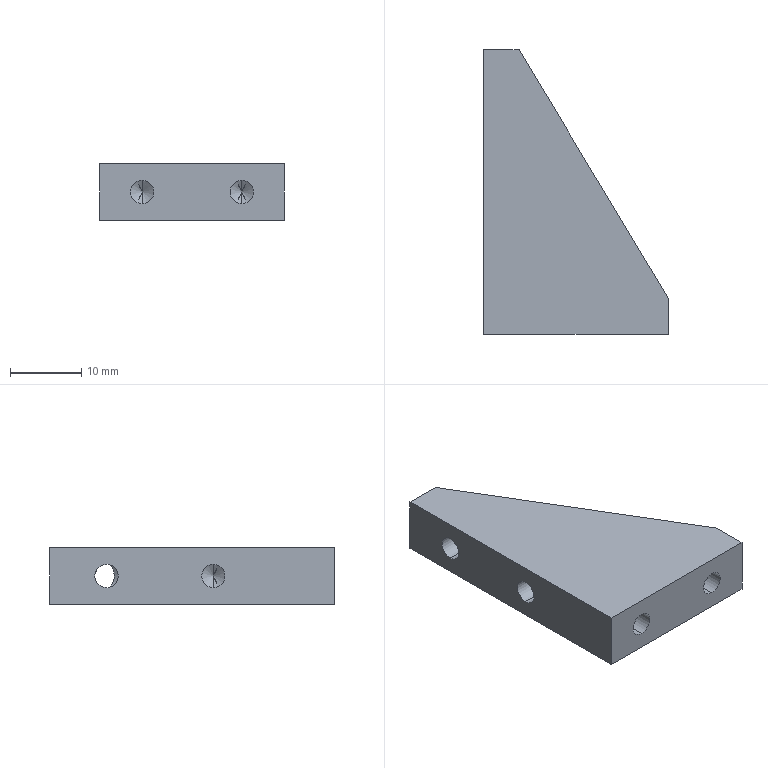Part | STEP file | FBDS-TL-006 | 1 solid | 22 faces | box 26 x 40 x 8 mm | volume 5029 mm3 | cylinder 8 | cone 7 | plane 7 | commonest cylinder face diameters 3.3 x8
STEP:
#1=CARTESIAN_POINT('',(20.,10.1,5.65));
#2=VERTEX_POINT('',#1);
#3=CARTESIAN_POINT('',(20.,10.1,2.35));
#4=VERTEX_POINT('',#3);
#5=CARTESIAN_POINT('',(20.,10.1,4.));
#6=DIRECTION('',(0.,-1.,0.));
#7=DIRECTION('',(0.,0.,-1.));
#8=AXIS2_PLACEMENT_3D('',#5,#6,#7);
#9=CIRCLE('',#8,1.65);
#10=EDGE_CURVE('',#2,#4,#9,.T.);
#11=ORIENTED_EDGE('',*,*,#10,.F.);
#12=CARTESIAN_POINT('',(20.,0.,5.65));
#13=VERTEX_POINT('',#12);
#14=CARTESIAN_POINT('',(20.,0.,5.65));
#15=DIRECTION('',(0.,-1.,0.));
#16=VECTOR('',#15,1000.);
#17=LINE('',#14,#16);
#18=EDGE_CURVE('',#2,#13,#17,.T.);
#19=ORIENTED_EDGE('',*,*,#18,.T.);
#20=CARTESIAN_POINT('',(20.,0.,2.35));
#21=VERTEX_POINT('',#20);
#22=CARTESIAN_POINT('',(20.,0.,4.));
#23=DIRECTION('',(0.,-1.,0.));
#24=DIRECTION('',(0.,0.,-1.));
#25=AXIS2_PLACEMENT_3D('',#22,#23,#24);
#26=CIRCLE('',#25,1.65);
#27=EDGE_CURVE('',#13,#21,#26,.T.);
#28=ORIENTED_EDGE('',*,*,#27,.T.);
#29=CARTESIAN_POINT('',(20.,0.,2.35));
#30=DIRECTION('',(0.,-1.,0.));
#31=VECTOR('',#30,1000.);
#32=LINE('',#29,#31);
#33=EDGE_CURVE('',#4,#21,#32,.T.);
#34=ORIENTED_EDGE('',*,*,#33,.F.);
#35=EDGE_LOOP('',(#11,#19,#28,#34));
#36=FACE_OUTER_BOUND('',#35,.T.);
#37=CARTESIAN_POINT('',(20.,0.,4.));
#38=DIRECTION('',(0.,-1.,0.));
#39=DIRECTION('',(0.,0.,-1.));
#40=AXIS2_PLACEMENT_3D('',#37,#38,#39);
#41=CYLINDRICAL_SURFACE('',#40,1.65);
#42=ADVANCED_FACE('',(#36),#41,.F.);
#43=CARTESIAN_POINT('',(20.,11.091,4.));
#44=VERTEX_POINT('',#43);
#45=CARTESIAN_POINT('',(20.,10.1,2.35));
#46=DIRECTION('',(0.,-0.515,-0.8572));
#47=VECTOR('',#46,1000.);
#48=LINE('',#45,#47);
#49=EDGE_CURVE('',#44,#4,#48,.T.);
#50=ORIENTED_EDGE('',*,*,#49,.F.);
#51=CARTESIAN_POINT('',(20.,10.1,5.65));
#52=DIRECTION('',(0.,-0.515,0.8572));
#53=VECTOR('',#52,1000.);
#54=LINE('',#51,#53);
#55=EDGE_CURVE('',#44,#2,#54,.T.);
#56=ORIENTED_EDGE('',*,*,#55,.T.);
#57=ORIENTED_EDGE('',*,*,#10,.T.);
#58=EDGE_LOOP('',(#50,#56,#57));
#59=FACE_OUTER_BOUND('',#58,.T.);
#60=CARTESIAN_POINT('',(20.,10.1,4.));
#61=DIRECTION('',(0.,-1.,0.));
#62=DIRECTION('',(0.,0.,-1.));
#63=AXIS2_PLACEMENT_3D('',#60,#61,#62);
#64=CONICAL_SURFACE('',#63,1.65,1.03);
#65=ADVANCED_FACE('',(#59),#64,.F.);
#66=CARTESIAN_POINT('',(6.,10.1,5.65));
#67=VERTEX_POINT('',#66);
#68=CARTESIAN_POINT('',(6.,10.1,2.35));
#69=VERTEX_POINT('',#68);
#70=CARTESIAN_POINT('',(6.,10.1,4.));
#71=DIRECTION('',(0.,-1.,0.));
#72=DIRECTION('',(0.,0.,-1.));
#73=AXIS2_PLACEMENT_3D('',#70,#71,#72);
#74=CIRCLE('',#73,1.65);
#75=EDGE_CURVE('',#67,#69,#74,.T.);
#76=ORIENTED_EDGE('',*,*,#75,.F.);
#77=CARTESIAN_POINT('',(6.,0.,5.65));
#78=VERTEX_POINT('',#77);
#79=CARTESIAN_POINT('',(6.,0.,5.65));
#80=DIRECTION('',(0.,-1.,0.));
#81=VECTOR('',#80,1000.);
#82=LINE('',#79,#81);
#83=EDGE_CURVE('',#67,#78,#82,.T.);
#84=ORIENTED_EDGE('',*,*,#83,.T.);
#85=CARTESIAN_POINT('',(6.,0.,2.35));
#86=VERTEX_POINT('',#85);
#87=CARTESIAN_POINT('',(6.,0.,4.));
#88=DIRECTION('',(0.,-1.,0.));
#89=DIRECTION('',(0.,0.,-1.));
#90=AXIS2_PLACEMENT_3D('',#87,#88,#89);
#91=CIRCLE('',#90,1.65);
#92=EDGE_CURVE('',#78,#86,#91,.T.);
#93=ORIENTED_EDGE('',*,*,#92,.T.);
#94=CARTESIAN_POINT('',(6.,0.,2.35));
#95=DIRECTION('',(0.,-1.,0.));
#96=VECTOR('',#95,1000.);
#97=LINE('',#94,#96);
#98=EDGE_CURVE('',#69,#86,#97,.T.);
#99=ORIENTED_EDGE('',*,*,#98,.F.);
#100=EDGE_LOOP('',(#76,#84,#93,#99));
#101=FACE_OUTER_BOUND('',#100,.T.);
#102=CARTESIAN_POINT('',(6.,0.,4.));
#103=DIRECTION('',(0.,-1.,0.));
#104=DIRECTION('',(0.,0.,-1.));
#105=AXIS2_PLACEMENT_3D('',#102,#103,#104);
#106=CYLINDRICAL_SURFACE('',#105,1.65);
#107=ADVANCED_FACE('',(#101),#106,.F.);
#108=CARTESIAN_POINT('',(6.,11.091,4.));
#109=VERTEX_POINT('',#108);
#110=CARTESIAN_POINT('',(6.,10.1,2.35));
#111=DIRECTION('',(0.,-0.515,-0.8572));
#112=VECTOR('',#111,1000.);
#113=LINE('',#110,#112);
#114=EDGE_CURVE('',#109,#69,#113,.T.);
#115=ORIENTED_EDGE('',*,*,#114,.F.);
#116=CARTESIAN_POINT('',(6.,10.1,5.65));
#117=DIRECTION('',(0.,-0.515,0.8572));
#118=VECTOR('',#117,1000.);
#119=LINE('',#116,#118);
#120=EDGE_CURVE('',#109,#67,#119,.T.);
#121=ORIENTED_EDGE('',*,*,#120,.T.);
#122=ORIENTED_EDGE('',*,*,#75,.T.);
#123=EDGE_LOOP('',(#115,#121,#122));
#124=FACE_OUTER_BOUND('',#123,.T.);
#125=CARTESIAN_POINT('',(6.,10.1,4.));
#126=DIRECTION('',(0.,-1.,0.));
#127=DIRECTION('',(0.,0.,-1.));
#128=AXIS2_PLACEMENT_3D('',#125,#126,#127);
#129=CONICAL_SURFACE('',#128,1.65,1.03);
#130=ADVANCED_FACE('',(#124),#129,.F.);
#131=CARTESIAN_POINT('',(9.8,32.,2.35));
#132=VERTEX_POINT('',#131);
#133=CARTESIAN_POINT('',(10.1,31.5,2.428));
#134=VERTEX_POINT('',#133);
#135=CARTESIAN_POINT('',(9.8,32.,2.35));
#136=CARTESIAN_POINT('',(9.902,31.83,2.35));
#137=CARTESIAN_POINT('',(10.003,31.662,2.376));
#138=CARTESIAN_POINT('',(10.1,31.5,2.428));
#139=(BOUNDED_CURVE()B_SPLINE_CURVE(3,(#135,#136,#137,#138),.UNSPECIFIED.,.F.,.F.)B_SPLINE_CURVE_WITH_KNOTS((4,4),(1.571,1.879),.UNSPECIFIED.)CURVE()GEOMETRIC_REPRESENTATION_ITEM()RATIONAL_B_SPLINE_CURVE((1.,0.9921,0.9921,1.))REPRESENTATION_ITEM(''));
#140=EDGE_CURVE('',#132,#134,#139,.T.);
#141=ORIENTED_EDGE('',*,*,#140,.F.);
#142=CARTESIAN_POINT('',(0.,32.,2.35));
#143=VERTEX_POINT('',#142);
#144=CARTESIAN_POINT('',(0.,32.,2.35));
#145=DIRECTION('',(-1.,0.,0.));
#146=VECTOR('',#145,1000.);
#147=LINE('',#144,#146);
#148=EDGE_CURVE('',#132,#143,#147,.T.);
#149=ORIENTED_EDGE('',*,*,#148,.T.);
#150=CARTESIAN_POINT('',(0.,32.,5.65));
#151=VERTEX_POINT('',#150);
#152=CARTESIAN_POINT('',(0.,32.,4.));
#153=DIRECTION('',(-1.,0.,0.));
#154=DIRECTION('',(0.,0.,1.));
#155=AXIS2_PLACEMENT_3D('',#152,#153,#154);
#156=CIRCLE('',#155,1.65);
#157=EDGE_CURVE('',#143,#151,#156,.T.);
#158=ORIENTED_EDGE('',*,*,#157,.T.);
#159=CARTESIAN_POINT('',(9.8,32.,5.65));
#160=VERTEX_POINT('',#159);
#161=CARTESIAN_POINT('',(0.,32.,5.65));
#162=DIRECTION('',(-1.,0.,0.));
#163=VECTOR('',#162,1000.);
#164=LINE('',#161,#163);
#165=EDGE_CURVE('',#160,#151,#164,.T.);
#166=ORIENTED_EDGE('',*,*,#165,.F.);
#167=CARTESIAN_POINT('',(10.1,31.5,5.572));
#168=VERTEX_POINT('',#167);
#169=CARTESIAN_POINT('',(10.1,31.5,5.572));
#170=CARTESIAN_POINT('',(10.003,31.662,5.624));
#171=CARTESIAN_POINT('',(9.902,31.83,5.65));
#172=CARTESIAN_POINT('',(9.8,32.,5.65));
#173=(BOUNDED_CURVE()B_SPLINE_CURVE(3,(#169,#170,#171,#172),.UNSPECIFIED.,.F.,.F.)B_SPLINE_CURVE_WITH_KNOTS((4,4),(4.405,4.712),.UNSPECIFIED.)CURVE()GEOMETRIC_REPRESENTATION_ITEM()RATIONAL_B_SPLINE_CURVE((1.,0.9921,0.9921,1.))REPRESENTATION_ITEM(''));
#174=EDGE_CURVE('',#168,#160,#173,.T.);
#175=ORIENTED_EDGE('',*,*,#174,.F.);
#176=CARTESIAN_POINT('',(10.1,32.,4.));
#177=DIRECTION('',(-1.,0.,0.));
#178=DIRECTION('',(0.,0.,1.));
#179=AXIS2_PLACEMENT_3D('',#176,#177,#178);
#180=CIRCLE('',#179,1.65);
#181=EDGE_CURVE('',#134,#168,#180,.T.);
#182=ORIENTED_EDGE('',*,*,#181,.F.);
#183=EDGE_LOOP('',(#141,#149,#158,#166,#175,#182));
#184=FACE_OUTER_BOUND('',#183,.T.);
#185=CARTESIAN_POINT('',(0.,32.,4.));
#186=DIRECTION('',(-1.,0.,0.));
#187=DIRECTION('',(0.,0.,1.));
#188=AXIS2_PLACEMENT_3D('',#185,#186,#187);
#189=CYLINDRICAL_SURFACE('',#188,1.65);
#190=ADVANCED_FACE('',(#184),#189,.F.);
#191=CARTESIAN_POINT('',(10.1,17.,2.35));
#192=VERTEX_POINT('',#191);
#193=CARTESIAN_POINT('',(10.1,17.,5.65));
#194=VERTEX_POINT('',#193);
#195=CARTESIAN_POINT('',(10.1,17.,4.));
#196=DIRECTION('',(-1.,0.,0.));
#197=DIRECTION('',(0.,0.,1.));
#198=AXIS2_PLACEMENT_3D('',#195,#196,#197);
#199=CIRCLE('',#198,1.65);
#200=EDGE_CURVE('',#192,#194,#199,.T.);
#201=ORIENTED_EDGE('',*,*,#200,.F.);
#202=CARTESIAN_POINT('',(0.,17.,2.35));
#203=VERTEX_POINT('',#202);
#204=CARTESIAN_POINT('',(0.,17.,2.35));
#205=DIRECTION('',(-1.,0.,0.));
#206=VECTOR('',#205,1000.);
#207=LINE('',#204,#206);
#208=EDGE_CURVE('',#192,#203,#207,.T.);
#209=ORIENTED_EDGE('',*,*,#208,.T.);
#210=CARTESIAN_POINT('',(0.,17.,5.65));
#211=VERTEX_POINT('',#210);
#212=CARTESIAN_POINT('',(0.,17.,4.));
#213=DIRECTION('',(-1.,0.,0.));
#214=DIRECTION('',(0.,0.,1.));
#215=AXIS2_PLACEMENT_3D('',#212,#213,#214);
#216=CIRCLE('',#215,1.65);
#217=EDGE_CURVE('',#203,#211,#216,.T.);
#218=ORIENTED_EDGE('',*,*,#217,.T.);
#219=CARTESIAN_POINT('',(0.,17.,5.65));
#220=DIRECTION('',(-1.,0.,0.));
#221=VECTOR('',#220,1000.);
#222=LINE('',#219,#221);
#223=EDGE_CURVE('',#194,#211,#222,.T.);
#224=ORIENTED_EDGE('',*,*,#223,.F.);
#225=EDGE_LOOP('',(#201,#209,#218,#224));
#226=FACE_OUTER_BOUND('',#225,.T.);
#227=CARTESIAN_POINT('',(0.,17.,4.));
#228=DIRECTION('',(-1.,0.,0.));
#229=DIRECTION('',(0.,0.,1.));
#230=AXIS2_PLACEMENT_3D('',#227,#228,#229);
#231=CYLINDRICAL_SURFACE('',#230,1.65);
#232=ADVANCED_FACE('',(#226),#231,.F.);
#233=CARTESIAN_POINT('',(11.091,17.,4.));
#234=VERTEX_POINT('',#233);
#235=CARTESIAN_POINT('',(10.1,17.,5.65));
#236=DIRECTION('',(-0.515,0.,0.8572));
#237=VECTOR('',#236,1000.);
#238=LINE('',#235,#237);
#239=EDGE_CURVE('',#234,#194,#238,.T.);
#240=ORIENTED_EDGE('',*,*,#239,.F.);
#241=CARTESIAN_POINT('',(10.1,17.,2.35));
#242=DIRECTION('',(-0.515,0.,-0.8572));
#243=VECTOR('',#242,1000.);
#244=LINE('',#241,#243);
#245=EDGE_CURVE('',#234,#192,#244,.T.);
#246=ORIENTED_EDGE('',*,*,#245,.T.);
#247=ORIENTED_EDGE('',*,*,#200,.T.);
#248=EDGE_LOOP('',(#240,#246,#247));
#249=FACE_OUTER_BOUND('',#248,.T.);
#250=CARTESIAN_POINT('',(10.1,17.,4.));
#251=DIRECTION('',(-1.,0.,0.));
#252=DIRECTION('',(0.,0.,1.));
#253=AXIS2_PLACEMENT_3D('',#250,#251,#252);
#254=CONICAL_SURFACE('',#253,1.65,1.03);
#255=ADVANCED_FACE('',(#249),#254,.F.);
#256=CARTESIAN_POINT('',(0.,32.,4.));
#257=DIRECTION('',(-1.,0.,0.));
#258=DIRECTION('',(0.,0.,1.));
#259=AXIS2_PLACEMENT_3D('',#256,#257,#258);
#260=CIRCLE('',#259,1.65);
#261=EDGE_CURVE('',#151,#143,#260,.T.);
#262=ORIENTED_EDGE('',*,*,#261,.F.);
#263=ORIENTED_EDGE('',*,*,#157,.F.);
#264=EDGE_LOOP('',(#262,#263));
#265=FACE_BOUND('',#264,.T.);
#266=CARTESIAN_POINT('',(0.,17.,4.));
#267=DIRECTION('',(-1.,0.,0.));
#268=DIRECTION('',(0.,0.,1.));
#269=AXIS2_PLACEMENT_3D('',#266,#267,#268);
#270=CIRCLE('',#269,1.65);
#271=EDGE_CURVE('',#211,#203,#270,.T.);
#272=ORIENTED_EDGE('',*,*,#271,.F.);
#273=ORIENTED_EDGE('',*,*,#217,.F.);
#274=EDGE_LOOP('',(#272,#273));
#275=FACE_BOUND('',#274,.T.);
#276=CARTESIAN_POINT('',(0.,40.,0.));
#277=VERTEX_POINT('',#276);
#278=CARTESIAN_POINT('',(0.,0.,0.));
#279=VERTEX_POINT('',#278);
#280=CARTESIAN_POINT('',(0.,40.,0.));
#281=DIRECTION('',(0.,-1.,0.));
#282=VECTOR('',#281,1000.);
#283=LINE('',#280,#282);
#284=EDGE_CURVE('',#277,#279,#283,.T.);
#285=ORIENTED_EDGE('',*,*,#284,.T.);
#286=CARTESIAN_POINT('',(0.,0.,8.));
#287=VERTEX_POINT('',#286);
#288=CARTESIAN_POINT('',(0.,0.,8.));
#289=DIRECTION('',(0.,0.,-1.));
#290=VECTOR('',#289,1000.);
#291=LINE('',#288,#290);
#292=EDGE_CURVE('',#287,#279,#291,.T.);
#293=ORIENTED_EDGE('',*,*,#292,.F.);
#294=CARTESIAN_POINT('',(0.,40.,8.));
#295=VERTEX_POINT('',#294);
#296=CARTESIAN_POINT('',(0.,40.,8.));
#297=DIRECTION('',(0.,-1.,0.));
#298=VECTOR('',#297,1000.);
#299=LINE('',#296,#298);
#300=EDGE_CURVE('',#295,#287,#299,.T.);
#301=ORIENTED_EDGE('',*,*,#300,.F.);
#302=CARTESIAN_POINT('',(0.,40.,8.));
#303=DIRECTION('',(0.,0.,-1.));
#304=VECTOR('',#303,1000.);
#305=LINE('',#302,#304);
#306=EDGE_CURVE('',#295,#277,#305,.T.);
#307=ORIENTED_EDGE('',*,*,#306,.T.);
#308=EDGE_LOOP('',(#285,#293,#301,#307));
#309=FACE_OUTER_BOUND('',#308,.T.);
#310=CARTESIAN_POINT('',(0.,40.,8.));
#311=DIRECTION('',(1.,0.,0.));
#312=DIRECTION('',(0.,1.,0.));
#313=AXIS2_PLACEMENT_3D('',#310,#311,#312);
#314=PLANE('',#313);
#315=ADVANCED_FACE('',(#265,#275,#309),#314,.F.);
#316=CARTESIAN_POINT('',(20.,0.,4.));
#317=DIRECTION('',(0.,-1.,0.));
#318=DIRECTION('',(0.,0.,-1.));
#319=AXIS2_PLACEMENT_3D('',#316,#317,#318);
#320=CIRCLE('',#319,1.65);
#321=EDGE_CURVE('',#21,#13,#320,.T.);
#322=ORIENTED_EDGE('',*,*,#321,.F.);
#323=ORIENTED_EDGE('',*,*,#27,.F.);
#324=EDGE_LOOP('',(#322,#323));
#325=FACE_BOUND('',#324,.T.);
#326=CARTESIAN_POINT('',(6.,0.,4.));
#327=DIRECTION('',(0.,-1.,0.));
#328=DIRECTION('',(0.,0.,-1.));
#329=AXIS2_PLACEMENT_3D('',#326,#327,#328);
#330=CIRCLE('',#329,1.65);
#331=EDGE_CURVE('',#86,#78,#330,.T.);
#332=ORIENTED_EDGE('',*,*,#331,.F.);
#333=ORIENTED_EDGE('',*,*,#92,.F.);
#334=EDGE_LOOP('',(#332,#333));
#335=FACE_BOUND('',#334,.T.);
#336=CARTESIAN_POINT('',(26.,0.,0.));
#337=VERTEX_POINT('',#336);
#338=CARTESIAN_POINT('',(0.,0.,0.));
#339=DIRECTION('',(1.,0.,0.));
#340=VECTOR('',#339,1000.);
#341=LINE('',#338,#340);
#342=EDGE_CURVE('',#279,#337,#341,.T.);
#343=ORIENTED_EDGE('',*,*,#342,.T.);
#344=CARTESIAN_POINT('',(26.,0.,8.));
#345=VERTEX_POINT('',#344);
#346=CARTESIAN_POINT('',(26.,0.,8.));
#347=DIRECTION('',(0.,0.,-1.));
#348=VECTOR('',#347,1000.);
#349=LINE('',#346,#348);
#350=EDGE_CURVE('',#345,#337,#349,.T.);
#351=ORIENTED_EDGE('',*,*,#350,.F.);
#352=CARTESIAN_POINT('',(0.,0.,8.));
#353=DIRECTION('',(1.,0.,0.));
#354=VECTOR('',#353,1000.);
#355=LINE('',#352,#354);
#356=EDGE_CURVE('',#287,#345,#355,.T.);
#357=ORIENTED_EDGE('',*,*,#356,.F.);
#358=ORIENTED_EDGE('',*,*,#292,.T.);
#359=EDGE_LOOP('',(#343,#351,#357,#358));
#360=FACE_OUTER_BOUND('',#359,.T.);
#361=CARTESIAN_POINT('',(0.,0.,8.));
#362=DIRECTION('',(0.,1.,0.));
#363=DIRECTION('',(0.,0.,1.));
#364=AXIS2_PLACEMENT_3D('',#361,#362,#363);
#365=PLANE('',#364);
#366=ADVANCED_FACE('',(#325,#335,#360),#365,.F.);
#367=CARTESIAN_POINT('',(26.,5.,0.));
#368=VERTEX_POINT('',#367);
#369=CARTESIAN_POINT('',(26.,0.,0.));
#370=DIRECTION('',(0.,1.,0.));
#371=VECTOR('',#370,1000.);
#372=LINE('',#369,#371);
#373=EDGE_CURVE('',#337,#368,#372,.T.);
#374=ORIENTED_EDGE('',*,*,#373,.T.);
#375=CARTESIAN_POINT('',(26.,5.,8.));
#376=VERTEX_POINT('',#375);
#377=CARTESIAN_POINT('',(26.,5.,8.));
#378=DIRECTION('',(0.,0.,-1.));
#379=VECTOR('',#378,1000.);
#380=LINE('',#377,#379);
#381=EDGE_CURVE('',#376,#368,#380,.T.);
#382=ORIENTED_EDGE('',*,*,#381,.F.);
#383=CARTESIAN_POINT('',(26.,0.,8.));
#384=DIRECTION('',(0.,1.,0.));
#385=VECTOR('',#384,1000.);
#386=LINE('',#383,#385);
#387=EDGE_CURVE('',#345,#376,#386,.T.);
#388=ORIENTED_EDGE('',*,*,#387,.F.);
#389=ORIENTED_EDGE('',*,*,#350,.T.);
#390=EDGE_LOOP('',(#374,#382,#388,#389));
#391=FACE_OUTER_BOUND('',#390,.T.);
#392=CARTESIAN_POINT('',(26.,0.,8.));
#393=DIRECTION('',(-1.,0.,0.));
#394=DIRECTION('',(0.,0.,1.));
#395=AXIS2_PLACEMENT_3D('',#392,#393,#394);
#396=PLANE('',#395);
#397=ADVANCED_FACE('',(#391),#396,.F.);
#398=CARTESIAN_POINT('',(10.1,31.5,2.428));
#399=CARTESIAN_POINT('',(10.56,30.733,3.476));
#400=CARTESIAN_POINT('',(10.56,30.733,4.524));
#401=CARTESIAN_POINT('',(10.1,31.5,5.572));
#402=(BOUNDED_CURVE()B_SPLINE_CURVE(3,(#398,#399,#400,#401),.UNSPECIFIED.,.F.,.F.)B_SPLINE_CURVE_WITH_KNOTS((4,4),(3.102,3.181),.UNSPECIFIED.)CURVE()GEOMETRIC_REPRESENTATION_ITEM()RATIONAL_B_SPLINE_CURVE((1.,0.9995,0.9995,1.))REPRESENTATION_ITEM(''));
#403=EDGE_CURVE('',#134,#168,#402,.T.);
#404=ORIENTED_EDGE('',*,*,#403,.T.);
#405=ORIENTED_EDGE('',*,*,#174,.T.);
#406=CARTESIAN_POINT('',(9.8,32.,5.65));
#407=CARTESIAN_POINT('',(7.82,35.3,5.65));
#408=CARTESIAN_POINT('',(7.82,35.3,2.35));
#409=CARTESIAN_POINT('',(9.8,32.,2.35));
#410=(BOUNDED_CURVE()B_SPLINE_CURVE(3,(#406,#407,#408,#409),.UNSPECIFIED.,.F.,.F.)B_SPLINE_CURVE_WITH_KNOTS((4,4),(4.712,7.854),.UNSPECIFIED.)CURVE()GEOMETRIC_REPRESENTATION_ITEM()RATIONAL_B_SPLINE_CURVE((1.,0.3333,0.3333,1.))REPRESENTATION_ITEM(''));
#411=EDGE_CURVE('',#160,#132,#410,.T.);
#412=ORIENTED_EDGE('',*,*,#411,.T.);
#413=ORIENTED_EDGE('',*,*,#140,.T.);
#414=EDGE_LOOP('',(#404,#405,#412,#413));
#415=FACE_BOUND('',#414,.T.);
#416=CARTESIAN_POINT('',(5.,40.,0.));
#417=VERTEX_POINT('',#416);
#418=CARTESIAN_POINT('',(26.,5.,0.));
#419=DIRECTION('',(-0.5145,0.8575,0.));
#420=VECTOR('',#419,1000.);
#421=LINE('',#418,#420);
#422=EDGE_CURVE('',#368,#417,#421,.T.);
#423=ORIENTED_EDGE('',*,*,#422,.T.);
#424=CARTESIAN_POINT('',(5.,40.,8.));
#425=VERTEX_POINT('',#424);
#426=CARTESIAN_POINT('',(5.,40.,8.));
#427=DIRECTION('',(0.,0.,-1.));
#428=VECTOR('',#427,1000.);
#429=LINE('',#426,#428);
#430=EDGE_CURVE('',#425,#417,#429,.T.);
#431=ORIENTED_EDGE('',*,*,#430,.F.);
#432=CARTESIAN_POINT('',(26.,5.,8.));
#433=DIRECTION('',(-0.5145,0.8575,0.));
#434=VECTOR('',#433,1000.);
#435=LINE('',#432,#434);
#436=EDGE_CURVE('',#376,#425,#435,.T.);
#437=ORIENTED_EDGE('',*,*,#436,.F.);
#438=ORIENTED_EDGE('',*,*,#381,.T.);
#439=EDGE_LOOP('',(#423,#431,#437,#438));
#440=FACE_OUTER_BOUND('',#439,.T.);
#441=CARTESIAN_POINT('',(26.,5.,8.));
#442=DIRECTION('',(-0.8575,-0.5145,0.));
#443=DIRECTION('',(0.5145,-0.8575,0.));
#444=AXIS2_PLACEMENT_3D('',#441,#442,#443);
#445=PLANE('',#444);
#446=ADVANCED_FACE('',(#415,#440),#445,.F.);
#447=CARTESIAN_POINT('',(5.,40.,0.));
#448=DIRECTION('',(-1.,0.,0.));
#449=VECTOR('',#448,1000.);
#450=LINE('',#447,#449);
#451=EDGE_CURVE('',#417,#277,#450,.T.);
#452=ORIENTED_EDGE('',*,*,#451,.T.);
#453=ORIENTED_EDGE('',*,*,#306,.F.);
#454=CARTESIAN_POINT('',(5.,40.,8.));
#455=DIRECTION('',(-1.,0.,0.));
#456=VECTOR('',#455,1000.);
#457=LINE('',#454,#456);
#458=EDGE_CURVE('',#425,#295,#457,.T.);
#459=ORIENTED_EDGE('',*,*,#458,.F.);
#460=ORIENTED_EDGE('',*,*,#430,.T.);
#461=EDGE_LOOP('',(#452,#453,#459,#460));
#462=FACE_OUTER_BOUND('',#461,.T.);
#463=CARTESIAN_POINT('',(5.,40.,8.));
#464=DIRECTION('',(0.,-1.,0.));
#465=DIRECTION('',(0.,0.,-1.));
#466=AXIS2_PLACEMENT_3D('',#463,#464,#465);
#467=PLANE('',#466);
#468=ADVANCED_FACE('',(#462),#467,.F.);
#469=ORIENTED_EDGE('',*,*,#300,.T.);
#470=ORIENTED_EDGE('',*,*,#356,.T.);
#471=ORIENTED_EDGE('',*,*,#387,.T.);
#472=ORIENTED_EDGE('',*,*,#436,.T.);
#473=ORIENTED_EDGE('',*,*,#458,.T.);
#474=EDGE_LOOP('',(#469,#470,#471,#472,#473));
#475=FACE_OUTER_BOUND('',#474,.T.);
#476=CARTESIAN_POINT('',(0.,0.,8.));
#477=DIRECTION('',(0.,0.,1.));
#478=DIRECTION('',(1.,0.,0.));
#479=AXIS2_PLACEMENT_3D('',#476,#477,#478);
#480=PLANE('',#479);
#481=ADVANCED_FACE('',(#475),#480,.T.);
#482=ORIENTED_EDGE('',*,*,#284,.F.);
#483=ORIENTED_EDGE('',*,*,#451,.F.);
#484=ORIENTED_EDGE('',*,*,#422,.F.);
#485=ORIENTED_EDGE('',*,*,#373,.F.);
#486=ORIENTED_EDGE('',*,*,#342,.F.);
#487=EDGE_LOOP('',(#482,#483,#484,#485,#486));
#488=FACE_OUTER_BOUND('',#487,.T.);
#489=CARTESIAN_POINT('',(0.,0.,0.));
#490=DIRECTION('',(0.,0.,1.));
#491=DIRECTION('',(1.,0.,0.));
#492=AXIS2_PLACEMENT_3D('',#489,#490,#491);
#493=PLANE('',#492);
#494=ADVANCED_FACE('',(#488),#493,.F.);
#495=ORIENTED_EDGE('',*,*,#245,.F.);
#496=ORIENTED_EDGE('',*,*,#239,.T.);
#497=CARTESIAN_POINT('',(10.1,17.,4.));
#498=DIRECTION('',(-1.,0.,0.));
#499=DIRECTION('',(0.,0.,1.));
#500=AXIS2_PLACEMENT_3D('',#497,#498,#499);
#501=CIRCLE('',#500,1.65);
#502=EDGE_CURVE('',#194,#192,#501,.T.);
#503=ORIENTED_EDGE('',*,*,#502,.T.);
#504=EDGE_LOOP('',(#495,#496,#503));
#505=FACE_OUTER_BOUND('',#504,.T.);
#506=CARTESIAN_POINT('',(10.1,17.,4.));
#507=DIRECTION('',(-1.,0.,0.));
#508=DIRECTION('',(0.,0.,1.));
#509=AXIS2_PLACEMENT_3D('',#506,#507,#508);
#510=CONICAL_SURFACE('',#509,1.65,1.03);
#511=ADVANCED_FACE('',(#505),#510,.F.);
#512=ORIENTED_EDGE('',*,*,#208,.F.);
#513=ORIENTED_EDGE('',*,*,#502,.F.);
#514=ORIENTED_EDGE('',*,*,#223,.T.);
#515=ORIENTED_EDGE('',*,*,#271,.T.);
#516=EDGE_LOOP('',(#512,#513,#514,#515));
#517=FACE_OUTER_BOUND('',#516,.T.);
#518=CARTESIAN_POINT('',(0.,17.,4.));
#519=DIRECTION('',(-1.,0.,0.));
#520=DIRECTION('',(0.,0.,1.));
#521=AXIS2_PLACEMENT_3D('',#518,#519,#520);
#522=CYLINDRICAL_SURFACE('',#521,1.65);
#523=ADVANCED_FACE('',(#517),#522,.F.);
#524=ORIENTED_EDGE('',*,*,#148,.F.);
#525=ORIENTED_EDGE('',*,*,#411,.F.);
#526=ORIENTED_EDGE('',*,*,#165,.T.);
#527=ORIENTED_EDGE('',*,*,#261,.T.);
#528=EDGE_LOOP('',(#524,#525,#526,#527));
#529=FACE_OUTER_BOUND('',#528,.T.);
#530=CARTESIAN_POINT('',(0.,32.,4.));
#531=DIRECTION('',(-1.,0.,0.));
#532=DIRECTION('',(0.,0.,1.));
#533=AXIS2_PLACEMENT_3D('',#530,#531,#532);
#534=CYLINDRICAL_SURFACE('',#533,1.65);
#535=ADVANCED_FACE('',(#529),#534,.F.);
#536=ORIENTED_EDGE('',*,*,#181,.T.);
#537=ORIENTED_EDGE('',*,*,#403,.F.);
#538=EDGE_LOOP('',(#536,#537));
#539=FACE_OUTER_BOUND('',#538,.T.);
#540=CARTESIAN_POINT('',(10.1,32.,4.));
#541=DIRECTION('',(-1.,0.,0.));
#542=DIRECTION('',(0.,0.,1.));
#543=AXIS2_PLACEMENT_3D('',#540,#541,#542);
#544=CONICAL_SURFACE('',#543,1.65,1.03);
#545=ADVANCED_FACE('',(#539),#544,.F.);
#546=ORIENTED_EDGE('',*,*,#120,.F.);
#547=ORIENTED_EDGE('',*,*,#114,.T.);
#548=CARTESIAN_POINT('',(6.,10.1,4.));
#549=DIRECTION('',(0.,-1.,0.));
#550=DIRECTION('',(0.,0.,-1.));
#551=AXIS2_PLACEMENT_3D('',#548,#549,#550);
#552=CIRCLE('',#551,1.65);
#553=EDGE_CURVE('',#69,#67,#552,.T.);
#554=ORIENTED_EDGE('',*,*,#553,.T.);
#555=EDGE_LOOP('',(#546,#547,#554));
#556=FACE_OUTER_BOUND('',#555,.T.);
#557=CARTESIAN_POINT('',(6.,10.1,4.));
#558=DIRECTION('',(0.,-1.,0.));
#559=DIRECTION('',(0.,0.,-1.));
#560=AXIS2_PLACEMENT_3D('',#557,#558,#559);
#561=CONICAL_SURFACE('',#560,1.65,1.03);
#562=ADVANCED_FACE('',(#556),#561,.F.);
#563=ORIENTED_EDGE('',*,*,#83,.F.);
#564=ORIENTED_EDGE('',*,*,#553,.F.);
#565=ORIENTED_EDGE('',*,*,#98,.T.);
#566=ORIENTED_EDGE('',*,*,#331,.T.);
#567=EDGE_LOOP('',(#563,#564,#565,#566));
#568=FACE_OUTER_BOUND('',#567,.T.);
#569=CARTESIAN_POINT('',(6.,0.,4.));
#570=DIRECTION('',(0.,-1.,0.));
#571=DIRECTION('',(0.,0.,-1.));
#572=AXIS2_PLACEMENT_3D('',#569,#570,#571);
#573=CYLINDRICAL_SURFACE('',#572,1.65);
#574=ADVANCED_FACE('',(#568),#573,.F.);
#575=ORIENTED_EDGE('',*,*,#55,.F.);
#576=ORIENTED_EDGE('',*,*,#49,.T.);
#577=CARTESIAN_POINT('',(20.,10.1,4.));
#578=DIRECTION('',(0.,-1.,0.));
#579=DIRECTION('',(0.,0.,-1.));
#580=AXIS2_PLACEMENT_3D('',#577,#578,#579);
#581=CIRCLE('',#580,1.65);
#582=EDGE_CURVE('',#4,#2,#581,.T.);
#583=ORIENTED_EDGE('',*,*,#582,.T.);
#584=EDGE_LOOP('',(#575,#576,#583));
#585=FACE_OUTER_BOUND('',#584,.T.);
#586=CARTESIAN_POINT('',(20.,10.1,4.));
#587=DIRECTION('',(0.,-1.,0.));
#588=DIRECTION('',(0.,0.,-1.));
#589=AXIS2_PLACEMENT_3D('',#586,#587,#588);
#590=CONICAL_SURFACE('',#589,1.65,1.03);
#591=ADVANCED_FACE('',(#585),#590,.F.);
#592=ORIENTED_EDGE('',*,*,#18,.F.);
#593=ORIENTED_EDGE('',*,*,#582,.F.);
#594=ORIENTED_EDGE('',*,*,#33,.T.);
#595=ORIENTED_EDGE('',*,*,#321,.T.);
#596=EDGE_LOOP('',(#592,#593,#594,#595));
#597=FACE_OUTER_BOUND('',#596,.T.);
#598=CARTESIAN_POINT('',(20.,0.,4.));
#599=DIRECTION('',(0.,-1.,0.));
#600=DIRECTION('',(0.,0.,-1.));
#601=AXIS2_PLACEMENT_3D('',#598,#599,#600);
#602=CYLINDRICAL_SURFACE('',#601,1.65);
#603=ADVANCED_FACE('',(#597),#602,.F.);
#604=CLOSED_SHELL('',(#42,#65,#107,#130,#190,#232,#255,#315,#366,#397,#446,#468,#481,#494,#511,#523,#535,#545,#562,#574,#591,#603));
#605=MANIFOLD_SOLID_BREP('',#604);
#606=CARTESIAN_POINT('',(0.,0.,0.));
#607=DIRECTION('',(0.,0.,1.));
#608=DIRECTION('',(1.,0.,0.));
#609=AXIS2_PLACEMENT_3D('',#606,#607,#608);
#610=(LENGTH_UNIT()NAMED_UNIT(*)SI_UNIT(.MILLI.,.METRE.));
#611=UNCERTAINTY_MEASURE_WITH_UNIT(LENGTH_MEASURE(0.00001),#610,'','');
#612=(NAMED_UNIT(*)PLANE_ANGLE_UNIT()SI_UNIT($,.RADIAN.));
#613=(NAMED_UNIT(*)SI_UNIT($,.STERADIAN.)SOLID_ANGLE_UNIT());
#614=(GEOMETRIC_REPRESENTATION_CONTEXT(3)GLOBAL_UNCERTAINTY_ASSIGNED_CONTEXT((#611))GLOBAL_UNIT_ASSIGNED_CONTEXT((#610,#612,#613))REPRESENTATION_CONTEXT('',''));
#615=ADVANCED_BREP_SHAPE_REPRESENTATION('',(#605,#609),#614);